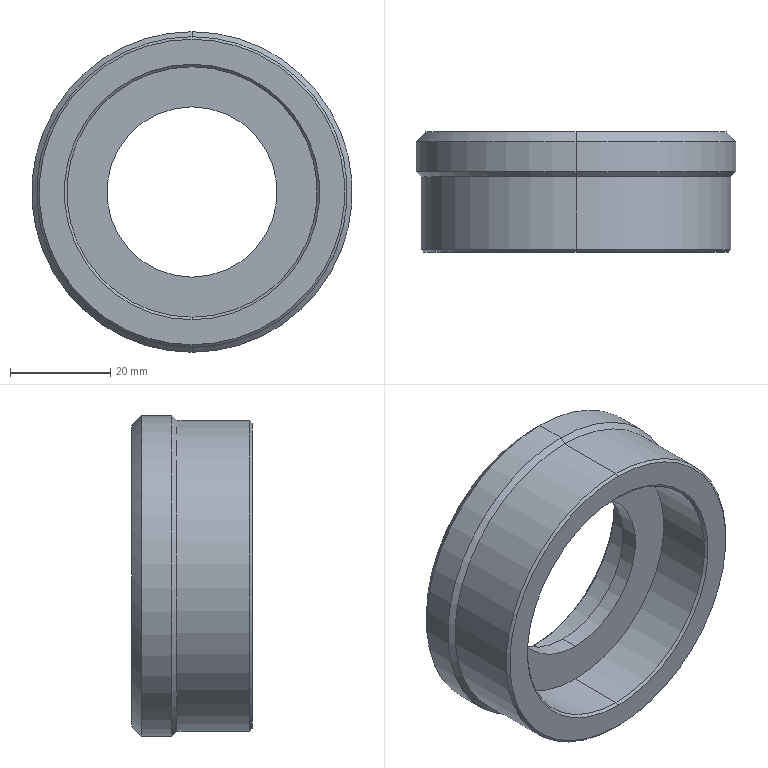Part | SolidWorks | features ICE 4, Chamfer 3, Extrusion 1, HoleWzd 1 | 1 solid | 32 faces | box 64 x 24 x 64 mm | volume 33265 mm3 | cone 14 | cylinder 14 | plane 4 | commonest cylinder face diameters 4 x4 34 x2 45 x2 50 x2 62 x2 64 x2
STEP:
#1=CARTESIAN_POINT('',(0.,15.,-31.));
#2=VERTEX_POINT('',#1);
#3=CARTESIAN_POINT('',(0.,15.,31.));
#4=VERTEX_POINT('',#3);
#5=CARTESIAN_POINT('',(0.,15.,0.));
#6=DIRECTION('',(0.,-1.,0.));
#7=DIRECTION('',(0.,0.,1.));
#8=AXIS2_PLACEMENT_3D('',#5,#6,#7);
#9=CIRCLE('',#8,31.);
#10=EDGE_CURVE('',#2,#4,#9,.T.);
#11=ORIENTED_EDGE('',*,*,#10,.F.);
#12=CARTESIAN_POINT('',(0.,16.,-32.));
#13=VERTEX_POINT('',#12);
#14=CARTESIAN_POINT('',(0.,16.,-32.));
#15=DIRECTION('',(0.,0.7071,-0.7071));
#16=VECTOR('',#15,1000.);
#17=LINE('',#14,#16);
#18=EDGE_CURVE('',#2,#13,#17,.T.);
#19=ORIENTED_EDGE('',*,*,#18,.T.);
#20=CARTESIAN_POINT('',(0.,16.,32.));
#21=VERTEX_POINT('',#20);
#22=CARTESIAN_POINT('',(0.,16.,0.));
#23=DIRECTION('',(0.,1.,0.));
#24=DIRECTION('',(0.,0.,1.));
#25=AXIS2_PLACEMENT_3D('',#22,#23,#24);
#26=CIRCLE('',#25,32.);
#27=EDGE_CURVE('',#21,#13,#26,.T.);
#28=ORIENTED_EDGE('',*,*,#27,.F.);
#29=CARTESIAN_POINT('',(0.,16.,32.));
#30=DIRECTION('',(0.,0.7071,0.7071));
#31=VECTOR('',#30,1000.);
#32=LINE('',#29,#31);
#33=EDGE_CURVE('',#4,#21,#32,.T.);
#34=ORIENTED_EDGE('',*,*,#33,.F.);
#35=EDGE_LOOP('',(#11,#19,#28,#34));
#36=FACE_OUTER_BOUND('',#35,.T.);
#37=CARTESIAN_POINT('',(0.,16.,0.));
#38=DIRECTION('',(0.,1.,0.));
#39=DIRECTION('',(0.,0.,1.));
#40=AXIS2_PLACEMENT_3D('',#37,#38,#39);
#41=CONICAL_SURFACE('',#40,32.,0.7854);
#42=ADVANCED_FACE('',(#36),#41,.T.);
#43=CARTESIAN_POINT('',(0.,24.,30.));
#44=VERTEX_POINT('',#43);
#45=CARTESIAN_POINT('',(0.,24.,-30.));
#46=VERTEX_POINT('',#45);
#47=CARTESIAN_POINT('',(0.,24.,0.));
#48=DIRECTION('',(0.,1.,0.));
#49=DIRECTION('',(0.,0.,1.));
#50=AXIS2_PLACEMENT_3D('',#47,#48,#49);
#51=CIRCLE('',#50,30.);
#52=EDGE_CURVE('',#44,#46,#51,.T.);
#53=ORIENTED_EDGE('',*,*,#52,.F.);
#54=CARTESIAN_POINT('',(0.,22.,32.));
#55=VERTEX_POINT('',#54);
#56=CARTESIAN_POINT('',(0.,24.,30.));
#57=DIRECTION('',(0.,-0.7071,0.7071));
#58=VECTOR('',#57,1000.);
#59=LINE('',#56,#58);
#60=EDGE_CURVE('',#44,#55,#59,.T.);
#61=ORIENTED_EDGE('',*,*,#60,.T.);
#62=CARTESIAN_POINT('',(0.,22.,-32.));
#63=VERTEX_POINT('',#62);
#64=CARTESIAN_POINT('',(0.,22.,0.));
#65=DIRECTION('',(0.,-1.,0.));
#66=DIRECTION('',(0.,0.,1.));
#67=AXIS2_PLACEMENT_3D('',#64,#65,#66);
#68=CIRCLE('',#67,32.);
#69=EDGE_CURVE('',#63,#55,#68,.T.);
#70=ORIENTED_EDGE('',*,*,#69,.F.);
#71=CARTESIAN_POINT('',(0.,24.,-30.));
#72=DIRECTION('',(0.,-0.7071,-0.7071));
#73=VECTOR('',#72,1000.);
#74=LINE('',#71,#73);
#75=EDGE_CURVE('',#46,#63,#74,.T.);
#76=ORIENTED_EDGE('',*,*,#75,.F.);
#77=EDGE_LOOP('',(#53,#61,#70,#76));
#78=FACE_OUTER_BOUND('',#77,.T.);
#79=CARTESIAN_POINT('',(0.,24.,0.));
#80=DIRECTION('',(0.,-1.,0.));
#81=DIRECTION('',(0.,0.,-1.));
#82=AXIS2_PLACEMENT_3D('',#79,#80,#81);
#83=CONICAL_SURFACE('',#82,30.,0.7854);
#84=ADVANCED_FACE('',(#78),#83,.T.);
#85=ORIENTED_EDGE('',*,*,#27,.T.);
#86=CARTESIAN_POINT('',(0.,14.,-32.));
#87=DIRECTION('',(0.,1.,0.));
#88=VECTOR('',#87,1000.);
#89=LINE('',#86,#88);
#90=EDGE_CURVE('',#13,#63,#89,.T.);
#91=ORIENTED_EDGE('',*,*,#90,.T.);
#92=ORIENTED_EDGE('',*,*,#69,.T.);
#93=CARTESIAN_POINT('',(0.,14.,32.));
#94=DIRECTION('',(0.,1.,0.));
#95=VECTOR('',#94,1000.);
#96=LINE('',#93,#95);
#97=EDGE_CURVE('',#21,#55,#96,.T.);
#98=ORIENTED_EDGE('',*,*,#97,.F.);
#99=EDGE_LOOP('',(#85,#91,#92,#98));
#100=FACE_OUTER_BOUND('',#99,.T.);
#101=CARTESIAN_POINT('',(0.,14.,0.));
#102=DIRECTION('',(0.,1.,0.));
#103=DIRECTION('',(0.,0.,1.));
#104=AXIS2_PLACEMENT_3D('',#101,#102,#103);
#105=CYLINDRICAL_SURFACE('',#104,32.);
#106=ADVANCED_FACE('',(#100),#105,.T.);
#107=CARTESIAN_POINT('',(0.,18.,-29.5));
#108=VERTEX_POINT('',#107);
#109=CARTESIAN_POINT('',(0.,18.,-25.5));
#110=VERTEX_POINT('',#109);
#111=CARTESIAN_POINT('',(0.,18.,-27.5));
#112=DIRECTION('',(0.,1.,0.));
#113=DIRECTION('',(0.,0.,1.));
#114=AXIS2_PLACEMENT_3D('',#111,#112,#113);
#115=CIRCLE('',#114,2.);
#116=EDGE_CURVE('',#108,#110,#115,.T.);
#117=ORIENTED_EDGE('',*,*,#116,.F.);
#118=CARTESIAN_POINT('',(0.,24.,-29.5));
#119=VERTEX_POINT('',#118);
#120=CARTESIAN_POINT('',(0.,24.,-29.5));
#121=DIRECTION('',(0.,1.,0.));
#122=VECTOR('',#121,1000.);
#123=LINE('',#120,#122);
#124=EDGE_CURVE('',#108,#119,#123,.T.);
#125=ORIENTED_EDGE('',*,*,#124,.T.);
#126=CARTESIAN_POINT('',(0.,24.,-25.5));
#127=VERTEX_POINT('',#126);
#128=CARTESIAN_POINT('',(0.,24.,-27.5));
#129=DIRECTION('',(0.,1.,0.));
#130=DIRECTION('',(0.,0.,1.));
#131=AXIS2_PLACEMENT_3D('',#128,#129,#130);
#132=CIRCLE('',#131,2.);
#133=EDGE_CURVE('',#119,#127,#132,.T.);
#134=ORIENTED_EDGE('',*,*,#133,.T.);
#135=CARTESIAN_POINT('',(0.,24.,-25.5));
#136=DIRECTION('',(0.,1.,0.));
#137=VECTOR('',#136,1000.);
#138=LINE('',#135,#137);
#139=EDGE_CURVE('',#110,#127,#138,.T.);
#140=ORIENTED_EDGE('',*,*,#139,.F.);
#141=EDGE_LOOP('',(#117,#125,#134,#140));
#142=FACE_OUTER_BOUND('',#141,.T.);
#143=CARTESIAN_POINT('',(0.,24.,-27.5));
#144=DIRECTION('',(0.,1.,0.));
#145=DIRECTION('',(0.,0.,1.));
#146=AXIS2_PLACEMENT_3D('',#143,#144,#145);
#147=CYLINDRICAL_SURFACE('',#146,2.);
#148=ADVANCED_FACE('',(#142),#147,.F.);
#149=CARTESIAN_POINT('',(0.,16.798,-27.5));
#150=VERTEX_POINT('',#149);
#151=CARTESIAN_POINT('',(0.,18.,-25.5));
#152=DIRECTION('',(0.,0.515,0.8572));
#153=VECTOR('',#152,1000.);
#154=LINE('',#151,#153);
#155=EDGE_CURVE('',#150,#110,#154,.T.);
#156=ORIENTED_EDGE('',*,*,#155,.F.);
#157=CARTESIAN_POINT('',(0.,18.,-29.5));
#158=DIRECTION('',(0.,0.515,-0.8572));
#159=VECTOR('',#158,1000.);
#160=LINE('',#157,#159);
#161=EDGE_CURVE('',#150,#108,#160,.T.);
#162=ORIENTED_EDGE('',*,*,#161,.T.);
#163=ORIENTED_EDGE('',*,*,#116,.T.);
#164=EDGE_LOOP('',(#156,#162,#163));
#165=FACE_OUTER_BOUND('',#164,.T.);
#166=CARTESIAN_POINT('',(0.,18.,-27.5));
#167=DIRECTION('',(0.,1.,0.));
#168=DIRECTION('',(0.,0.,1.));
#169=AXIS2_PLACEMENT_3D('',#166,#167,#168);
#170=CONICAL_SURFACE('',#169,2.,1.03);
#171=ADVANCED_FACE('',(#165),#170,.F.);
#172=CARTESIAN_POINT('',(0.,18.,25.5));
#173=VERTEX_POINT('',#172);
#174=CARTESIAN_POINT('',(0.,18.,29.5));
#175=VERTEX_POINT('',#174);
#176=CARTESIAN_POINT('',(0.,18.,27.5));
#177=DIRECTION('',(0.,1.,0.));
#178=DIRECTION('',(0.,0.,1.));
#179=AXIS2_PLACEMENT_3D('',#176,#177,#178);
#180=CIRCLE('',#179,2.);
#181=EDGE_CURVE('',#173,#175,#180,.T.);
#182=ORIENTED_EDGE('',*,*,#181,.F.);
#183=CARTESIAN_POINT('',(0.,24.,25.5));
#184=VERTEX_POINT('',#183);
#185=CARTESIAN_POINT('',(0.,24.,25.5));
#186=DIRECTION('',(0.,1.,0.));
#187=VECTOR('',#186,1000.);
#188=LINE('',#185,#187);
#189=EDGE_CURVE('',#173,#184,#188,.T.);
#190=ORIENTED_EDGE('',*,*,#189,.T.);
#191=CARTESIAN_POINT('',(0.,24.,29.5));
#192=VERTEX_POINT('',#191);
#193=CARTESIAN_POINT('',(0.,24.,27.5));
#194=DIRECTION('',(0.,1.,0.));
#195=DIRECTION('',(0.,0.,1.));
#196=AXIS2_PLACEMENT_3D('',#193,#194,#195);
#197=CIRCLE('',#196,2.);
#198=EDGE_CURVE('',#184,#192,#197,.T.);
#199=ORIENTED_EDGE('',*,*,#198,.T.);
#200=CARTESIAN_POINT('',(0.,24.,29.5));
#201=DIRECTION('',(0.,1.,0.));
#202=VECTOR('',#201,1000.);
#203=LINE('',#200,#202);
#204=EDGE_CURVE('',#175,#192,#203,.T.);
#205=ORIENTED_EDGE('',*,*,#204,.F.);
#206=EDGE_LOOP('',(#182,#190,#199,#205));
#207=FACE_OUTER_BOUND('',#206,.T.);
#208=CARTESIAN_POINT('',(0.,24.,27.5));
#209=DIRECTION('',(0.,1.,0.));
#210=DIRECTION('',(0.,0.,1.));
#211=AXIS2_PLACEMENT_3D('',#208,#209,#210);
#212=CYLINDRICAL_SURFACE('',#211,2.);
#213=ADVANCED_FACE('',(#207),#212,.F.);
#214=CARTESIAN_POINT('',(0.,16.798,27.5));
#215=VERTEX_POINT('',#214);
#216=CARTESIAN_POINT('',(0.,18.,29.5));
#217=DIRECTION('',(0.,0.515,0.8572));
#218=VECTOR('',#217,1000.);
#219=LINE('',#216,#218);
#220=EDGE_CURVE('',#215,#175,#219,.T.);
#221=ORIENTED_EDGE('',*,*,#220,.F.);
#222=CARTESIAN_POINT('',(0.,18.,25.5));
#223=DIRECTION('',(0.,0.515,-0.8572));
#224=VECTOR('',#223,1000.);
#225=LINE('',#222,#224);
#226=EDGE_CURVE('',#215,#173,#225,.T.);
#227=ORIENTED_EDGE('',*,*,#226,.T.);
#228=ORIENTED_EDGE('',*,*,#181,.T.);
#229=EDGE_LOOP('',(#221,#227,#228));
#230=FACE_OUTER_BOUND('',#229,.T.);
#231=CARTESIAN_POINT('',(0.,18.,27.5));
#232=DIRECTION('',(0.,1.,0.));
#233=DIRECTION('',(0.,0.,1.));
#234=AXIS2_PLACEMENT_3D('',#231,#232,#233);
#235=CONICAL_SURFACE('',#234,2.,1.03);
#236=ADVANCED_FACE('',(#230),#235,.F.);
#237=CARTESIAN_POINT('',(0.,0.,-30.5));
#238=VERTEX_POINT('',#237);
#239=CARTESIAN_POINT('',(0.,0.,30.5));
#240=VERTEX_POINT('',#239);
#241=CARTESIAN_POINT('',(0.,0.,0.));
#242=DIRECTION('',(0.,-1.,0.));
#243=DIRECTION('',(0.,0.,1.));
#244=AXIS2_PLACEMENT_3D('',#241,#242,#243);
#245=CIRCLE('',#244,30.5);
#246=EDGE_CURVE('',#238,#240,#245,.T.);
#247=ORIENTED_EDGE('',*,*,#246,.F.);
#248=CARTESIAN_POINT('',(0.,0.5,-31.));
#249=VERTEX_POINT('',#248);
#250=CARTESIAN_POINT('',(0.,0.5,-31.));
#251=DIRECTION('',(0.,0.7071,-0.7071));
#252=VECTOR('',#251,1000.);
#253=LINE('',#250,#252);
#254=EDGE_CURVE('',#238,#249,#253,.T.);
#255=ORIENTED_EDGE('',*,*,#254,.T.);
#256=CARTESIAN_POINT('',(0.,0.5,31.));
#257=VERTEX_POINT('',#256);
#258=CARTESIAN_POINT('',(0.,0.5,0.));
#259=DIRECTION('',(0.,1.,0.));
#260=DIRECTION('',(0.,0.,1.));
#261=AXIS2_PLACEMENT_3D('',#258,#259,#260);
#262=CIRCLE('',#261,31.);
#263=EDGE_CURVE('',#257,#249,#262,.T.);
#264=ORIENTED_EDGE('',*,*,#263,.F.);
#265=CARTESIAN_POINT('',(0.,0.5,31.));
#266=DIRECTION('',(0.,0.7071,0.7071));
#267=VECTOR('',#266,1000.);
#268=LINE('',#265,#267);
#269=EDGE_CURVE('',#240,#257,#268,.T.);
#270=ORIENTED_EDGE('',*,*,#269,.F.);
#271=EDGE_LOOP('',(#247,#255,#264,#270));
#272=FACE_OUTER_BOUND('',#271,.T.);
#273=CARTESIAN_POINT('',(0.,0.5,0.));
#274=DIRECTION('',(0.,1.,0.));
#275=DIRECTION('',(0.,0.,1.));
#276=AXIS2_PLACEMENT_3D('',#273,#274,#275);
#277=CONICAL_SURFACE('',#276,31.,0.7854);
#278=ADVANCED_FACE('',(#272),#277,.T.);
#279=CARTESIAN_POINT('',(0.,0.5,25.));
#280=VERTEX_POINT('',#279);
#281=CARTESIAN_POINT('',(0.,0.5,-25.));
#282=VERTEX_POINT('',#281);
#283=CARTESIAN_POINT('',(0.,0.5,0.));
#284=DIRECTION('',(0.,-1.,0.));
#285=DIRECTION('',(0.,0.,1.));
#286=AXIS2_PLACEMENT_3D('',#283,#284,#285);
#287=CIRCLE('',#286,25.);
#288=EDGE_CURVE('',#280,#282,#287,.T.);
#289=ORIENTED_EDGE('',*,*,#288,.F.);
#290=CARTESIAN_POINT('',(0.,0.,25.5));
#291=VERTEX_POINT('',#290);
#292=CARTESIAN_POINT('',(0.,0.5,25.));
#293=DIRECTION('',(0.,-0.7071,0.7071));
#294=VECTOR('',#293,1000.);
#295=LINE('',#292,#294);
#296=EDGE_CURVE('',#280,#291,#295,.T.);
#297=ORIENTED_EDGE('',*,*,#296,.T.);
#298=CARTESIAN_POINT('',(0.,0.,-25.5));
#299=VERTEX_POINT('',#298);
#300=CARTESIAN_POINT('',(0.,0.,0.));
#301=DIRECTION('',(0.,1.,0.));
#302=DIRECTION('',(0.,0.,1.));
#303=AXIS2_PLACEMENT_3D('',#300,#301,#302);
#304=CIRCLE('',#303,25.5);
#305=EDGE_CURVE('',#299,#291,#304,.T.);
#306=ORIENTED_EDGE('',*,*,#305,.F.);
#307=CARTESIAN_POINT('',(0.,0.5,-25.));
#308=DIRECTION('',(0.,-0.7071,-0.7071));
#309=VECTOR('',#308,1000.);
#310=LINE('',#307,#309);
#311=EDGE_CURVE('',#282,#299,#310,.T.);
#312=ORIENTED_EDGE('',*,*,#311,.F.);
#313=EDGE_LOOP('',(#289,#297,#306,#312));
#314=FACE_OUTER_BOUND('',#313,.T.);
#315=CARTESIAN_POINT('',(0.,0.5,0.));
#316=DIRECTION('',(0.,-1.,0.));
#317=DIRECTION('',(0.,0.,-1.));
#318=AXIS2_PLACEMENT_3D('',#315,#316,#317);
#319=CONICAL_SURFACE('',#318,25.,0.7854);
#320=ADVANCED_FACE('',(#314),#319,.F.);
#321=CARTESIAN_POINT('',(0.,23.5,-22.5));
#322=VERTEX_POINT('',#321);
#323=CARTESIAN_POINT('',(0.,23.5,22.5));
#324=VERTEX_POINT('',#323);
#325=CARTESIAN_POINT('',(0.,23.5,0.));
#326=DIRECTION('',(0.,1.,0.));
#327=DIRECTION('',(0.,0.,1.));
#328=AXIS2_PLACEMENT_3D('',#325,#326,#327);
#329=CIRCLE('',#328,22.5);
#330=EDGE_CURVE('',#322,#324,#329,.T.);
#331=ORIENTED_EDGE('',*,*,#330,.F.);
#332=CARTESIAN_POINT('',(0.,24.,-23.));
#333=VERTEX_POINT('',#332);
#334=CARTESIAN_POINT('',(0.,23.5,-22.5));
#335=DIRECTION('',(0.,0.7071,-0.7071));
#336=VECTOR('',#335,1000.);
#337=LINE('',#334,#336);
#338=EDGE_CURVE('',#322,#333,#337,.T.);
#339=ORIENTED_EDGE('',*,*,#338,.T.);
#340=CARTESIAN_POINT('',(0.,24.,23.));
#341=VERTEX_POINT('',#340);
#342=CARTESIAN_POINT('',(0.,24.,0.));
#343=DIRECTION('',(0.,-1.,0.));
#344=DIRECTION('',(0.,0.,1.));
#345=AXIS2_PLACEMENT_3D('',#342,#343,#344);
#346=CIRCLE('',#345,23.);
#347=EDGE_CURVE('',#341,#333,#346,.T.);
#348=ORIENTED_EDGE('',*,*,#347,.F.);
#349=CARTESIAN_POINT('',(0.,23.5,22.5));
#350=DIRECTION('',(0.,0.7071,0.7071));
#351=VECTOR('',#350,1000.);
#352=LINE('',#349,#351);
#353=EDGE_CURVE('',#324,#341,#352,.T.);
#354=ORIENTED_EDGE('',*,*,#353,.F.);
#355=EDGE_LOOP('',(#331,#339,#348,#354));
#356=FACE_OUTER_BOUND('',#355,.T.);
#357=CARTESIAN_POINT('',(0.,23.5,0.));
#358=DIRECTION('',(0.,1.,0.));
#359=DIRECTION('',(0.,0.,1.));
#360=AXIS2_PLACEMENT_3D('',#357,#358,#359);
#361=CONICAL_SURFACE('',#360,22.5,0.7854);
#362=ADVANCED_FACE('',(#356),#361,.F.);
#363=CARTESIAN_POINT('',(0.,12.,17.));
#364=VERTEX_POINT('',#363);
#365=CARTESIAN_POINT('',(0.,12.,-17.));
#366=VERTEX_POINT('',#365);
#367=CARTESIAN_POINT('',(0.,12.,0.));
#368=DIRECTION('',(0.,-1.,0.));
#369=DIRECTION('',(0.,0.,-1.));
#370=AXIS2_PLACEMENT_3D('',#367,#368,#369);
#371=CIRCLE('',#370,17.);
#372=EDGE_CURVE('',#364,#366,#371,.T.);
#373=ORIENTED_EDGE('',*,*,#372,.T.);
#374=CARTESIAN_POINT('',(0.,15.5,-17.));
#375=VERTEX_POINT('',#374);
#376=CARTESIAN_POINT('',(0.,0.,-17.));
#377=DIRECTION('',(0.,1.,0.));
#378=VECTOR('',#377,1000.);
#379=LINE('',#376,#378);
#380=EDGE_CURVE('',#366,#375,#379,.T.);
#381=ORIENTED_EDGE('',*,*,#380,.T.);
#382=CARTESIAN_POINT('',(0.,15.5,17.));
#383=VERTEX_POINT('',#382);
#384=CARTESIAN_POINT('',(0.,15.5,0.));
#385=DIRECTION('',(0.,1.,0.));
#386=DIRECTION('',(0.,0.,1.));
#387=AXIS2_PLACEMENT_3D('',#384,#385,#386);
#388=CIRCLE('',#387,17.);
#389=EDGE_CURVE('',#375,#383,#388,.T.);
#390=ORIENTED_EDGE('',*,*,#389,.T.);
#391=CARTESIAN_POINT('',(0.,0.,17.));
#392=DIRECTION('',(0.,1.,0.));
#393=VECTOR('',#392,1000.);
#394=LINE('',#391,#393);
#395=EDGE_CURVE('',#364,#383,#394,.T.);
#396=ORIENTED_EDGE('',*,*,#395,.F.);
#397=EDGE_LOOP('',(#373,#381,#390,#396));
#398=FACE_OUTER_BOUND('',#397,.T.);
#399=CARTESIAN_POINT('',(0.,0.,0.));
#400=DIRECTION('',(0.,1.,0.));
#401=DIRECTION('',(0.,0.,1.));
#402=AXIS2_PLACEMENT_3D('',#399,#400,#401);
#403=CYLINDRICAL_SURFACE('',#402,17.);
#404=ADVANCED_FACE('',(#398),#403,.F.);
#405=CARTESIAN_POINT('',(0.,15.5,-22.5));
#406=VERTEX_POINT('',#405);
#407=CARTESIAN_POINT('',(0.,15.5,22.5));
#408=VERTEX_POINT('',#407);
#409=CARTESIAN_POINT('',(0.,15.5,0.));
#410=DIRECTION('',(0.,1.,0.));
#411=DIRECTION('',(0.,0.,1.));
#412=AXIS2_PLACEMENT_3D('',#409,#410,#411);
#413=CIRCLE('',#412,22.5);
#414=EDGE_CURVE('',#406,#408,#413,.T.);
#415=ORIENTED_EDGE('',*,*,#414,.F.);
#416=CARTESIAN_POINT('',(0.,15.5,-22.5));
#417=DIRECTION('',(0.,1.,0.));
#418=VECTOR('',#417,1000.);
#419=LINE('',#416,#418);
#420=EDGE_CURVE('',#406,#322,#419,.T.);
#421=ORIENTED_EDGE('',*,*,#420,.T.);
#422=ORIENTED_EDGE('',*,*,#330,.T.);
#423=CARTESIAN_POINT('',(0.,15.5,22.5));
#424=DIRECTION('',(0.,1.,0.));
#425=VECTOR('',#424,1000.);
#426=LINE('',#423,#425);
#427=EDGE_CURVE('',#408,#324,#426,.T.);
#428=ORIENTED_EDGE('',*,*,#427,.F.);
#429=EDGE_LOOP('',(#415,#421,#422,#428));
#430=FACE_OUTER_BOUND('',#429,.T.);
#431=CARTESIAN_POINT('',(0.,15.5,0.));
#432=DIRECTION('',(0.,1.,0.));
#433=DIRECTION('',(0.,0.,1.));
#434=AXIS2_PLACEMENT_3D('',#431,#432,#433);
#435=CYLINDRICAL_SURFACE('',#434,22.5);
#436=ADVANCED_FACE('',(#430),#435,.F.);
#437=CARTESIAN_POINT('',(0.,12.,25.));
#438=VERTEX_POINT('',#437);
#439=CARTESIAN_POINT('',(0.,12.,-25.));
#440=VERTEX_POINT('',#439);
#441=CARTESIAN_POINT('',(0.,12.,0.));
#442=DIRECTION('',(0.,-1.,0.));
#443=DIRECTION('',(0.,0.,-1.));
#444=AXIS2_PLACEMENT_3D('',#441,#442,#443);
#445=CIRCLE('',#444,25.);
#446=EDGE_CURVE('',#438,#440,#445,.T.);
#447=ORIENTED_EDGE('',*,*,#446,.F.);
#448=CARTESIAN_POINT('',(0.,12.,25.));
#449=DIRECTION('',(0.,-1.,0.));
#450=VECTOR('',#449,1000.);
#451=LINE('',#448,#450);
#452=EDGE_CURVE('',#438,#280,#451,.T.);
#453=ORIENTED_EDGE('',*,*,#452,.T.);
#454=ORIENTED_EDGE('',*,*,#288,.T.);
#455=CARTESIAN_POINT('',(0.,12.,-25.));
#456=DIRECTION('',(0.,-1.,0.));
#457=VECTOR('',#456,1000.);
#458=LINE('',#455,#457);
#459=EDGE_CURVE('',#440,#282,#458,.T.);
#460=ORIENTED_EDGE('',*,*,#459,.F.);
#461=EDGE_LOOP('',(#447,#453,#454,#460));
#462=FACE_OUTER_BOUND('',#461,.T.);
#463=CARTESIAN_POINT('',(0.,12.,0.));
#464=DIRECTION('',(0.,-1.,0.));
#465=DIRECTION('',(0.,0.,-1.));
#466=AXIS2_PLACEMENT_3D('',#463,#464,#465);
#467=CYLINDRICAL_SURFACE('',#466,25.);
#468=ADVANCED_FACE('',(#462),#467,.F.);
#469=ORIENTED_EDGE('',*,*,#10,.T.);
#470=CARTESIAN_POINT('',(0.,24.,31.));
#471=DIRECTION('',(0.,-1.,0.));
#472=VECTOR('',#471,1000.);
#473=LINE('',#470,#472);
#474=EDGE_CURVE('',#4,#257,#473,.T.);
#475=ORIENTED_EDGE('',*,*,#474,.T.);
#476=ORIENTED_EDGE('',*,*,#263,.T.);
#477=CARTESIAN_POINT('',(0.,24.,-31.));
#478=DIRECTION('',(0.,-1.,0.));
#479=VECTOR('',#478,1000.);
#480=LINE('',#477,#479);
#481=EDGE_CURVE('',#2,#249,#480,.T.);
#482=ORIENTED_EDGE('',*,*,#481,.F.);
#483=EDGE_LOOP('',(#469,#475,#476,#482));
#484=FACE_OUTER_BOUND('',#483,.T.);
#485=CARTESIAN_POINT('',(0.,24.,0.));
#486=DIRECTION('',(0.,-1.,0.));
#487=DIRECTION('',(0.,0.,-1.));
#488=AXIS2_PLACEMENT_3D('',#485,#486,#487);
#489=CYLINDRICAL_SURFACE('',#488,31.);
#490=ADVANCED_FACE('',(#484),#489,.T.);
#491=ORIENTED_EDGE('',*,*,#474,.F.);
#492=CARTESIAN_POINT('',(0.,15.,0.));
#493=DIRECTION('',(0.,-1.,0.));
#494=DIRECTION('',(0.,0.,1.));
#495=AXIS2_PLACEMENT_3D('',#492,#493,#494);
#496=CIRCLE('',#495,31.);
#497=EDGE_CURVE('',#4,#2,#496,.T.);
#498=ORIENTED_EDGE('',*,*,#497,.T.);
#499=ORIENTED_EDGE('',*,*,#481,.T.);
#500=CARTESIAN_POINT('',(0.,0.5,0.));
#501=DIRECTION('',(0.,1.,0.));
#502=DIRECTION('',(0.,0.,1.));
#503=AXIS2_PLACEMENT_3D('',#500,#501,#502);
#504=CIRCLE('',#503,31.);
#505=EDGE_CURVE('',#249,#257,#504,.T.);
#506=ORIENTED_EDGE('',*,*,#505,.T.);
#507=EDGE_LOOP('',(#491,#498,#499,#506));
#508=FACE_OUTER_BOUND('',#507,.T.);
#509=CARTESIAN_POINT('',(0.,24.,0.));
#510=DIRECTION('',(0.,-1.,0.));
#511=DIRECTION('',(0.,0.,-1.));
#512=AXIS2_PLACEMENT_3D('',#509,#510,#511);
#513=CYLINDRICAL_SURFACE('',#512,31.);
#514=ADVANCED_FACE('',(#508),#513,.T.);
#515=CARTESIAN_POINT('',(0.,24.,0.));
#516=DIRECTION('',(0.,1.,0.));
#517=DIRECTION('',(0.,0.,1.));
#518=AXIS2_PLACEMENT_3D('',#515,#516,#517);
#519=CIRCLE('',#518,30.);
#520=EDGE_CURVE('',#46,#44,#519,.T.);
#521=ORIENTED_EDGE('',*,*,#520,.T.);
#522=ORIENTED_EDGE('',*,*,#52,.T.);
#523=EDGE_LOOP('',(#521,#522));
#524=FACE_OUTER_BOUND('',#523,.T.);
#525=CARTESIAN_POINT('',(0.,24.,-27.5));
#526=DIRECTION('',(0.,1.,0.));
#527=DIRECTION('',(0.,0.,1.));
#528=AXIS2_PLACEMENT_3D('',#525,#526,#527);
#529=CIRCLE('',#528,2.);
#530=EDGE_CURVE('',#127,#119,#529,.T.);
#531=ORIENTED_EDGE('',*,*,#530,.F.);
#532=ORIENTED_EDGE('',*,*,#133,.F.);
#533=EDGE_LOOP('',(#531,#532));
#534=FACE_BOUND('',#533,.T.);
#535=CARTESIAN_POINT('',(0.,24.,27.5));
#536=DIRECTION('',(0.,1.,0.));
#537=DIRECTION('',(0.,0.,1.));
#538=AXIS2_PLACEMENT_3D('',#535,#536,#537);
#539=CIRCLE('',#538,2.);
#540=EDGE_CURVE('',#192,#184,#539,.T.);
#541=ORIENTED_EDGE('',*,*,#540,.F.);
#542=ORIENTED_EDGE('',*,*,#198,.F.);
#543=EDGE_LOOP('',(#541,#542));
#544=FACE_BOUND('',#543,.T.);
#545=ORIENTED_EDGE('',*,*,#347,.T.);
#546=CARTESIAN_POINT('',(0.,24.,0.));
#547=DIRECTION('',(0.,-1.,0.));
#548=DIRECTION('',(0.,0.,1.));
#549=AXIS2_PLACEMENT_3D('',#546,#547,#548);
#550=CIRCLE('',#549,23.);
#551=EDGE_CURVE('',#333,#341,#550,.T.);
#552=ORIENTED_EDGE('',*,*,#551,.T.);
#553=EDGE_LOOP('',(#545,#552));
#554=FACE_BOUND('',#553,.T.);
#555=CARTESIAN_POINT('',(0.,24.,0.));
#556=DIRECTION('',(0.,1.,0.));
#557=DIRECTION('',(0.,0.,1.));
#558=AXIS2_PLACEMENT_3D('',#555,#556,#557);
#559=PLANE('',#558);
#560=ADVANCED_FACE('',(#524,#534,#544,#554),#559,.T.);
#561=CARTESIAN_POINT('',(0.,0.,0.));
#562=DIRECTION('',(0.,-1.,0.));
#563=DIRECTION('',(0.,0.,1.));
#564=AXIS2_PLACEMENT_3D('',#561,#562,#563);
#565=CIRCLE('',#564,30.5);
#566=EDGE_CURVE('',#240,#238,#565,.T.);
#567=ORIENTED_EDGE('',*,*,#566,.T.);
#568=ORIENTED_EDGE('',*,*,#246,.T.);
#569=EDGE_LOOP('',(#567,#568));
#570=FACE_OUTER_BOUND('',#569,.T.);
#571=ORIENTED_EDGE('',*,*,#305,.T.);
#572=CARTESIAN_POINT('',(0.,0.,0.));
#573=DIRECTION('',(0.,1.,0.));
#574=DIRECTION('',(0.,0.,1.));
#575=AXIS2_PLACEMENT_3D('',#572,#573,#574);
#576=CIRCLE('',#575,25.5);
#577=EDGE_CURVE('',#291,#299,#576,.T.);
#578=ORIENTED_EDGE('',*,*,#577,.T.);
#579=EDGE_LOOP('',(#571,#578));
#580=FACE_BOUND('',#579,.T.);
#581=CARTESIAN_POINT('',(0.,0.,0.));
#582=DIRECTION('',(0.,1.,0.));
#583=DIRECTION('',(0.,0.,1.));
#584=AXIS2_PLACEMENT_3D('',#581,#582,#583);
#585=PLANE('',#584);
#586=ADVANCED_FACE('',(#570,#580),#585,.F.);
#587=ORIENTED_EDGE('',*,*,#452,.F.);
#588=CARTESIAN_POINT('',(0.,12.,0.));
#589=DIRECTION('',(0.,-1.,0.));
#590=DIRECTION('',(0.,0.,-1.));
#591=AXIS2_PLACEMENT_3D('',#588,#589,#590);
#592=CIRCLE('',#591,25.);
#593=EDGE_CURVE('',#440,#438,#592,.T.);
#594=ORIENTED_EDGE('',*,*,#593,.F.);
#595=ORIENTED_EDGE('',*,*,#459,.T.);
#596=CARTESIAN_POINT('',(0.,0.5,0.));
#597=DIRECTION('',(0.,-1.,0.));
#598=DIRECTION('',(0.,0.,1.));
#599=AXIS2_PLACEMENT_3D('',#596,#597,#598);
#600=CIRCLE('',#599,25.);
#601=EDGE_CURVE('',#282,#280,#600,.T.);
#602=ORIENTED_EDGE('',*,*,#601,.T.);
#603=EDGE_LOOP('',(#587,#594,#595,#602));
#604=FACE_OUTER_BOUND('',#603,.T.);
#605=CARTESIAN_POINT('',(0.,12.,0.));
#606=DIRECTION('',(0.,-1.,0.));
#607=DIRECTION('',(0.,0.,-1.));
#608=AXIS2_PLACEMENT_3D('',#605,#606,#607);
#609=CYLINDRICAL_SURFACE('',#608,25.);
#610=ADVANCED_FACE('',(#604),#609,.F.);
#611=ORIENTED_EDGE('',*,*,#372,.F.);
#612=CARTESIAN_POINT('',(0.,12.,0.));
#613=DIRECTION('',(0.,-1.,0.));
#614=DIRECTION('',(0.,0.,-1.));
#615=AXIS2_PLACEMENT_3D('',#612,#613,#614);
#616=CIRCLE('',#615,17.);
#617=EDGE_CURVE('',#366,#364,#616,.T.);
#618=ORIENTED_EDGE('',*,*,#617,.F.);
#619=EDGE_LOOP('',(#611,#618));
#620=FACE_BOUND('',#619,.T.);
#621=ORIENTED_EDGE('',*,*,#593,.T.);
#622=ORIENTED_EDGE('',*,*,#446,.T.);
#623=EDGE_LOOP('',(#621,#622));
#624=FACE_OUTER_BOUND('',#623,.T.);
#625=CARTESIAN_POINT('',(0.,12.,0.));
#626=DIRECTION('',(0.,-1.,0.));
#627=DIRECTION('',(0.,0.,-1.));
#628=AXIS2_PLACEMENT_3D('',#625,#626,#627);
#629=PLANE('',#628);
#630=ADVANCED_FACE('',(#620,#624),#629,.T.);
#631=ORIENTED_EDGE('',*,*,#420,.F.);
#632=CARTESIAN_POINT('',(0.,15.5,0.));
#633=DIRECTION('',(0.,1.,0.));
#634=DIRECTION('',(0.,0.,1.));
#635=AXIS2_PLACEMENT_3D('',#632,#633,#634);
#636=CIRCLE('',#635,22.5);
#637=EDGE_CURVE('',#408,#406,#636,.T.);
#638=ORIENTED_EDGE('',*,*,#637,.F.);
#639=ORIENTED_EDGE('',*,*,#427,.T.);
#640=CARTESIAN_POINT('',(0.,23.5,0.));
#641=DIRECTION('',(0.,1.,0.));
#642=DIRECTION('',(0.,0.,1.));
#643=AXIS2_PLACEMENT_3D('',#640,#641,#642);
#644=CIRCLE('',#643,22.5);
#645=EDGE_CURVE('',#324,#322,#644,.T.);
#646=ORIENTED_EDGE('',*,*,#645,.T.);
#647=EDGE_LOOP('',(#631,#638,#639,#646));
#648=FACE_OUTER_BOUND('',#647,.T.);
#649=CARTESIAN_POINT('',(0.,15.5,0.));
#650=DIRECTION('',(0.,1.,0.));
#651=DIRECTION('',(0.,0.,1.));
#652=AXIS2_PLACEMENT_3D('',#649,#650,#651);
#653=CYLINDRICAL_SURFACE('',#652,22.5);
#654=ADVANCED_FACE('',(#648),#653,.F.);
#655=CARTESIAN_POINT('',(0.,15.5,0.));
#656=DIRECTION('',(0.,1.,0.));
#657=DIRECTION('',(0.,0.,1.));
#658=AXIS2_PLACEMENT_3D('',#655,#656,#657);
#659=CIRCLE('',#658,17.);
#660=EDGE_CURVE('',#383,#375,#659,.T.);
#661=ORIENTED_EDGE('',*,*,#660,.F.);
#662=ORIENTED_EDGE('',*,*,#389,.F.);
#663=EDGE_LOOP('',(#661,#662));
#664=FACE_BOUND('',#663,.T.);
#665=ORIENTED_EDGE('',*,*,#637,.T.);
#666=ORIENTED_EDGE('',*,*,#414,.T.);
#667=EDGE_LOOP('',(#665,#666));
#668=FACE_OUTER_BOUND('',#667,.T.);
#669=CARTESIAN_POINT('',(0.,15.5,0.));
#670=DIRECTION('',(0.,1.,0.));
#671=DIRECTION('',(0.,0.,1.));
#672=AXIS2_PLACEMENT_3D('',#669,#670,#671);
#673=PLANE('',#672);
#674=ADVANCED_FACE('',(#664,#668),#673,.T.);
#675=ORIENTED_EDGE('',*,*,#380,.F.);
#676=ORIENTED_EDGE('',*,*,#617,.T.);
#677=ORIENTED_EDGE('',*,*,#395,.T.);
#678=ORIENTED_EDGE('',*,*,#660,.T.);
#679=EDGE_LOOP('',(#675,#676,#677,#678));
#680=FACE_OUTER_BOUND('',#679,.T.);
#681=CARTESIAN_POINT('',(0.,0.,0.));
#682=DIRECTION('',(0.,1.,0.));
#683=DIRECTION('',(0.,0.,1.));
#684=AXIS2_PLACEMENT_3D('',#681,#682,#683);
#685=CYLINDRICAL_SURFACE('',#684,17.);
#686=ADVANCED_FACE('',(#680),#685,.F.);
#687=ORIENTED_EDGE('',*,*,#338,.F.);
#688=ORIENTED_EDGE('',*,*,#645,.F.);
#689=ORIENTED_EDGE('',*,*,#353,.T.);
#690=ORIENTED_EDGE('',*,*,#551,.F.);
#691=EDGE_LOOP('',(#687,#688,#689,#690));
#692=FACE_OUTER_BOUND('',#691,.T.);
#693=CARTESIAN_POINT('',(0.,23.5,0.));
#694=DIRECTION('',(0.,1.,0.));
#695=DIRECTION('',(0.,0.,1.));
#696=AXIS2_PLACEMENT_3D('',#693,#694,#695);
#697=CONICAL_SURFACE('',#696,22.5,0.7854);
#698=ADVANCED_FACE('',(#692),#697,.F.);
#699=ORIENTED_EDGE('',*,*,#296,.F.);
#700=ORIENTED_EDGE('',*,*,#601,.F.);
#701=ORIENTED_EDGE('',*,*,#311,.T.);
#702=ORIENTED_EDGE('',*,*,#577,.F.);
#703=EDGE_LOOP('',(#699,#700,#701,#702));
#704=FACE_OUTER_BOUND('',#703,.T.);
#705=CARTESIAN_POINT('',(0.,0.5,0.));
#706=DIRECTION('',(0.,-1.,0.));
#707=DIRECTION('',(0.,0.,-1.));
#708=AXIS2_PLACEMENT_3D('',#705,#706,#707);
#709=CONICAL_SURFACE('',#708,25.,0.7854);
#710=ADVANCED_FACE('',(#704),#709,.F.);
#711=ORIENTED_EDGE('',*,*,#254,.F.);
#712=ORIENTED_EDGE('',*,*,#566,.F.);
#713=ORIENTED_EDGE('',*,*,#269,.T.);
#714=ORIENTED_EDGE('',*,*,#505,.F.);
#715=EDGE_LOOP('',(#711,#712,#713,#714));
#716=FACE_OUTER_BOUND('',#715,.T.);
#717=CARTESIAN_POINT('',(0.,0.5,0.));
#718=DIRECTION('',(0.,1.,0.));
#719=DIRECTION('',(0.,0.,1.));
#720=AXIS2_PLACEMENT_3D('',#717,#718,#719);
#721=CONICAL_SURFACE('',#720,31.,0.7854);
#722=ADVANCED_FACE('',(#716),#721,.T.);
#723=ORIENTED_EDGE('',*,*,#226,.F.);
#724=ORIENTED_EDGE('',*,*,#220,.T.);
#725=CARTESIAN_POINT('',(0.,18.,27.5));
#726=DIRECTION('',(0.,1.,0.));
#727=DIRECTION('',(0.,0.,1.));
#728=AXIS2_PLACEMENT_3D('',#725,#726,#727);
#729=CIRCLE('',#728,2.);
#730=EDGE_CURVE('',#175,#173,#729,.T.);
#731=ORIENTED_EDGE('',*,*,#730,.T.);
#732=EDGE_LOOP('',(#723,#724,#731));
#733=FACE_OUTER_BOUND('',#732,.T.);
#734=CARTESIAN_POINT('',(0.,18.,27.5));
#735=DIRECTION('',(0.,1.,0.));
#736=DIRECTION('',(0.,0.,1.));
#737=AXIS2_PLACEMENT_3D('',#734,#735,#736);
#738=CONICAL_SURFACE('',#737,2.,1.03);
#739=ADVANCED_FACE('',(#733),#738,.F.);
#740=ORIENTED_EDGE('',*,*,#189,.F.);
#741=ORIENTED_EDGE('',*,*,#730,.F.);
#742=ORIENTED_EDGE('',*,*,#204,.T.);
#743=ORIENTED_EDGE('',*,*,#540,.T.);
#744=EDGE_LOOP('',(#740,#741,#742,#743));
#745=FACE_OUTER_BOUND('',#744,.T.);
#746=CARTESIAN_POINT('',(0.,24.,27.5));
#747=DIRECTION('',(0.,1.,0.));
#748=DIRECTION('',(0.,0.,1.));
#749=AXIS2_PLACEMENT_3D('',#746,#747,#748);
#750=CYLINDRICAL_SURFACE('',#749,2.);
#751=ADVANCED_FACE('',(#745),#750,.F.);
#752=ORIENTED_EDGE('',*,*,#161,.F.);
#753=ORIENTED_EDGE('',*,*,#155,.T.);
#754=CARTESIAN_POINT('',(0.,18.,-27.5));
#755=DIRECTION('',(0.,1.,0.));
#756=DIRECTION('',(0.,0.,1.));
#757=AXIS2_PLACEMENT_3D('',#754,#755,#756);
#758=CIRCLE('',#757,2.);
#759=EDGE_CURVE('',#110,#108,#758,.T.);
#760=ORIENTED_EDGE('',*,*,#759,.T.);
#761=EDGE_LOOP('',(#752,#753,#760));
#762=FACE_OUTER_BOUND('',#761,.T.);
#763=CARTESIAN_POINT('',(0.,18.,-27.5));
#764=DIRECTION('',(0.,1.,0.));
#765=DIRECTION('',(0.,0.,1.));
#766=AXIS2_PLACEMENT_3D('',#763,#764,#765);
#767=CONICAL_SURFACE('',#766,2.,1.03);
#768=ADVANCED_FACE('',(#762),#767,.F.);
#769=ORIENTED_EDGE('',*,*,#124,.F.);
#770=ORIENTED_EDGE('',*,*,#759,.F.);
#771=ORIENTED_EDGE('',*,*,#139,.T.);
#772=ORIENTED_EDGE('',*,*,#530,.T.);
#773=EDGE_LOOP('',(#769,#770,#771,#772));
#774=FACE_OUTER_BOUND('',#773,.T.);
#775=CARTESIAN_POINT('',(0.,24.,-27.5));
#776=DIRECTION('',(0.,1.,0.));
#777=DIRECTION('',(0.,0.,1.));
#778=AXIS2_PLACEMENT_3D('',#775,#776,#777);
#779=CYLINDRICAL_SURFACE('',#778,2.);
#780=ADVANCED_FACE('',(#774),#779,.F.);
#781=ORIENTED_EDGE('',*,*,#90,.F.);
#782=CARTESIAN_POINT('',(0.,16.,0.));
#783=DIRECTION('',(0.,1.,0.));
#784=DIRECTION('',(0.,0.,1.));
#785=AXIS2_PLACEMENT_3D('',#782,#783,#784);
#786=CIRCLE('',#785,32.);
#787=EDGE_CURVE('',#13,#21,#786,.T.);
#788=ORIENTED_EDGE('',*,*,#787,.T.);
#789=ORIENTED_EDGE('',*,*,#97,.T.);
#790=CARTESIAN_POINT('',(0.,22.,0.));
#791=DIRECTION('',(0.,-1.,0.));
#792=DIRECTION('',(0.,0.,1.));
#793=AXIS2_PLACEMENT_3D('',#790,#791,#792);
#794=CIRCLE('',#793,32.);
#795=EDGE_CURVE('',#55,#63,#794,.T.);
#796=ORIENTED_EDGE('',*,*,#795,.T.);
#797=EDGE_LOOP('',(#781,#788,#789,#796));
#798=FACE_OUTER_BOUND('',#797,.T.);
#799=CARTESIAN_POINT('',(0.,14.,0.));
#800=DIRECTION('',(0.,1.,0.));
#801=DIRECTION('',(0.,0.,1.));
#802=AXIS2_PLACEMENT_3D('',#799,#800,#801);
#803=CYLINDRICAL_SURFACE('',#802,32.);
#804=ADVANCED_FACE('',(#798),#803,.T.);
#805=ORIENTED_EDGE('',*,*,#60,.F.);
#806=ORIENTED_EDGE('',*,*,#520,.F.);
#807=ORIENTED_EDGE('',*,*,#75,.T.);
#808=ORIENTED_EDGE('',*,*,#795,.F.);
#809=EDGE_LOOP('',(#805,#806,#807,#808));
#810=FACE_OUTER_BOUND('',#809,.T.);
#811=CARTESIAN_POINT('',(0.,24.,0.));
#812=DIRECTION('',(0.,-1.,0.));
#813=DIRECTION('',(0.,0.,-1.));
#814=AXIS2_PLACEMENT_3D('',#811,#812,#813);
#815=CONICAL_SURFACE('',#814,30.,0.7854);
#816=ADVANCED_FACE('',(#810),#815,.T.);
#817=ORIENTED_EDGE('',*,*,#18,.F.);
#818=ORIENTED_EDGE('',*,*,#497,.F.);
#819=ORIENTED_EDGE('',*,*,#33,.T.);
#820=ORIENTED_EDGE('',*,*,#787,.F.);
#821=EDGE_LOOP('',(#817,#818,#819,#820));
#822=FACE_OUTER_BOUND('',#821,.T.);
#823=CARTESIAN_POINT('',(0.,16.,0.));
#824=DIRECTION('',(0.,1.,0.));
#825=DIRECTION('',(0.,0.,1.));
#826=AXIS2_PLACEMENT_3D('',#823,#824,#825);
#827=CONICAL_SURFACE('',#826,32.,0.7854);
#828=ADVANCED_FACE('',(#822),#827,.T.);
#829=CLOSED_SHELL('',(#42,#84,#106,#148,#171,#213,#236,#278,#320,#362,#404,#436,#468,#490,#514,#560,#586,#610,#630,#654,#674,#686,#698,#710,#722,#739,#751,#768,#780,#804,#816,#828));
#830=MANIFOLD_SOLID_BREP('',#829);
#831=CARTESIAN_POINT('',(0.,0.,0.));
#832=DIRECTION('',(0.,0.,1.));
#833=DIRECTION('',(1.,0.,0.));
#834=AXIS2_PLACEMENT_3D('',#831,#832,#833);
#835=(LENGTH_UNIT()NAMED_UNIT(*)SI_UNIT(.MILLI.,.METRE.));
#836=UNCERTAINTY_MEASURE_WITH_UNIT(LENGTH_MEASURE(0.00001),#835,'','');
#837=(NAMED_UNIT(*)PLANE_ANGLE_UNIT()SI_UNIT($,.RADIAN.));
#838=(NAMED_UNIT(*)SI_UNIT($,.STERADIAN.)SOLID_ANGLE_UNIT());
#839=(GEOMETRIC_REPRESENTATION_CONTEXT(3)GLOBAL_UNCERTAINTY_ASSIGNED_CONTEXT((#836))GLOBAL_UNIT_ASSIGNED_CONTEXT((#835,#837,#838))REPRESENTATION_CONTEXT('',''));
#840=ADVANCED_BREP_SHAPE_REPRESENTATION('',(#830,#834),#839);